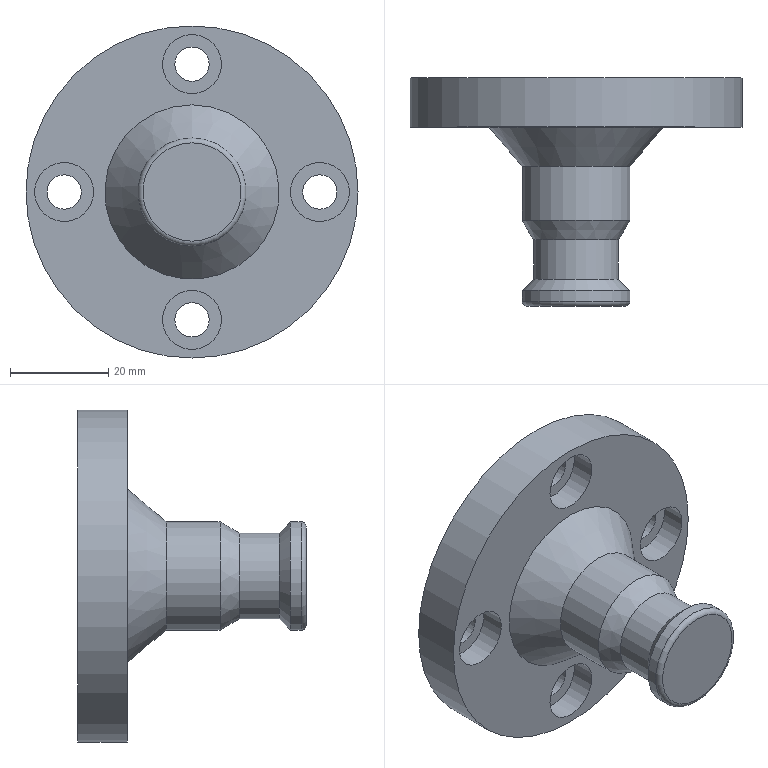Part | STEP file | Clamping device rod | 1 solid | 23 faces | box 67.5 x 46.39 x 67.5 mm | volume 47194 mm3 | cylinder 12 | plane 7 | cone 3 | torus 1 | commonest cylinder face diameters 7 x4 12 x4 22 x2 17.381 x1 67.5 x1
STEP:
#1=CARTESIAN_POINT('',(0.,38.89,-33.75));
#2=VERTEX_POINT('',#1);
#3=CARTESIAN_POINT('',(0.,38.89,0.));
#4=DIRECTION('',(0.,1.,0.));
#5=DIRECTION('',(0.,0.,-1.));
#6=AXIS2_PLACEMENT_3D('',#3,#4,#5);
#7=CIRCLE('',#6,33.75);
#8=EDGE_CURVE('',#2,#2,#7,.T.);
#9=ORIENTED_EDGE('',*,*,#8,.F.);
#10=EDGE_LOOP('',(#9));
#11=FACE_BOUND('',#10,.T.);
#12=CARTESIAN_POINT('',(26.,38.89,-6.));
#13=VERTEX_POINT('',#12);
#14=CARTESIAN_POINT('',(26.,38.89,0.));
#15=DIRECTION('',(0.,-1.,0.));
#16=DIRECTION('',(0.,0.,-1.));
#17=AXIS2_PLACEMENT_3D('',#14,#15,#16);
#18=CIRCLE('',#17,6.);
#19=EDGE_CURVE('',#13,#13,#18,.F.);
#20=ORIENTED_EDGE('',*,*,#19,.T.);
#21=EDGE_LOOP('',(#20));
#22=FACE_BOUND('',#21,.T.);
#23=CARTESIAN_POINT('',(-6.,38.89,-26.));
#24=VERTEX_POINT('',#23);
#25=CARTESIAN_POINT('',(0.,38.89,-26.));
#26=DIRECTION('',(0.,-1.,0.));
#27=DIRECTION('',(-1.,0.,0.));
#28=AXIS2_PLACEMENT_3D('',#25,#26,#27);
#29=CIRCLE('',#28,6.);
#30=EDGE_CURVE('',#24,#24,#29,.F.);
#31=ORIENTED_EDGE('',*,*,#30,.T.);
#32=EDGE_LOOP('',(#31));
#33=FACE_BOUND('',#32,.T.);
#34=CARTESIAN_POINT('',(-26.,38.89,6.));
#35=VERTEX_POINT('',#34);
#36=CARTESIAN_POINT('',(-26.,38.89,0.));
#37=DIRECTION('',(0.,-1.,0.));
#38=DIRECTION('',(0.,0.,1.));
#39=AXIS2_PLACEMENT_3D('',#36,#37,#38);
#40=CIRCLE('',#39,6.);
#41=EDGE_CURVE('',#35,#35,#40,.F.);
#42=ORIENTED_EDGE('',*,*,#41,.T.);
#43=EDGE_LOOP('',(#42));
#44=FACE_BOUND('',#43,.T.);
#45=CARTESIAN_POINT('',(0.,38.89,17.713));
#46=VERTEX_POINT('',#45);
#47=CARTESIAN_POINT('',(0.,38.89,0.));
#48=DIRECTION('',(0.,1.,0.));
#49=DIRECTION('',(0.,0.,1.));
#50=AXIS2_PLACEMENT_3D('',#47,#48,#49);
#51=CIRCLE('',#50,17.713);
#52=EDGE_CURVE('',#46,#46,#51,.T.);
#53=ORIENTED_EDGE('',*,*,#52,.T.);
#54=EDGE_LOOP('',(#53));
#55=FACE_BOUND('',#54,.T.);
#56=CARTESIAN_POINT('',(6.,38.89,26.));
#57=VERTEX_POINT('',#56);
#58=CARTESIAN_POINT('',(0.,38.89,26.));
#59=DIRECTION('',(0.,-1.,0.));
#60=DIRECTION('',(1.,0.,0.));
#61=AXIS2_PLACEMENT_3D('',#58,#59,#60);
#62=CIRCLE('',#61,6.);
#63=EDGE_CURVE('',#57,#57,#62,.F.);
#64=ORIENTED_EDGE('',*,*,#63,.T.);
#65=EDGE_LOOP('',(#64));
#66=FACE_BOUND('',#65,.T.);
#67=CARTESIAN_POINT('',(0.,38.89,0.));
#68=DIRECTION('',(0.,-1.,0.));
#69=DIRECTION('',(0.,0.,1.));
#70=AXIS2_PLACEMENT_3D('',#67,#68,#69);
#71=PLANE('',#70);
#72=ADVANCED_FACE('',(#11,#22,#33,#44,#55,#66),#71,.T.);
#73=CARTESIAN_POINT('',(0.,48.89,-33.75));
#74=VERTEX_POINT('',#73);
#75=CARTESIAN_POINT('',(0.,48.89,0.));
#76=DIRECTION('',(0.,1.,0.));
#77=DIRECTION('',(0.,0.,-1.));
#78=AXIS2_PLACEMENT_3D('',#75,#76,#77);
#79=CIRCLE('',#78,33.75);
#80=EDGE_CURVE('',#74,#74,#79,.T.);
#81=ORIENTED_EDGE('',*,*,#80,.T.);
#82=EDGE_LOOP('',(#81));
#83=FACE_BOUND('',#82,.T.);
#84=CARTESIAN_POINT('',(26.,48.89,-3.5));
#85=VERTEX_POINT('',#84);
#86=CARTESIAN_POINT('',(26.,48.89,0.));
#87=DIRECTION('',(0.,-1.,0.));
#88=DIRECTION('',(0.,0.,-1.));
#89=AXIS2_PLACEMENT_3D('',#86,#87,#88);
#90=CIRCLE('',#89,3.5);
#91=EDGE_CURVE('',#85,#85,#90,.T.);
#92=ORIENTED_EDGE('',*,*,#91,.T.);
#93=EDGE_LOOP('',(#92));
#94=FACE_BOUND('',#93,.T.);
#95=CARTESIAN_POINT('',(-3.5,48.89,-26.));
#96=VERTEX_POINT('',#95);
#97=CARTESIAN_POINT('',(0.,48.89,-26.));
#98=DIRECTION('',(0.,-1.,0.));
#99=DIRECTION('',(-1.,0.,0.));
#100=AXIS2_PLACEMENT_3D('',#97,#98,#99);
#101=CIRCLE('',#100,3.5);
#102=EDGE_CURVE('',#96,#96,#101,.T.);
#103=ORIENTED_EDGE('',*,*,#102,.T.);
#104=EDGE_LOOP('',(#103));
#105=FACE_BOUND('',#104,.T.);
#106=CARTESIAN_POINT('',(-26.,48.89,3.5));
#107=VERTEX_POINT('',#106);
#108=CARTESIAN_POINT('',(-26.,48.89,0.));
#109=DIRECTION('',(0.,-1.,0.));
#110=DIRECTION('',(0.,0.,1.));
#111=AXIS2_PLACEMENT_3D('',#108,#109,#110);
#112=CIRCLE('',#111,3.5);
#113=EDGE_CURVE('',#107,#107,#112,.T.);
#114=ORIENTED_EDGE('',*,*,#113,.T.);
#115=EDGE_LOOP('',(#114));
#116=FACE_BOUND('',#115,.T.);
#117=CARTESIAN_POINT('',(3.5,48.89,26.));
#118=VERTEX_POINT('',#117);
#119=CARTESIAN_POINT('',(0.,48.89,26.));
#120=DIRECTION('',(0.,-1.,0.));
#121=DIRECTION('',(1.,0.,0.));
#122=AXIS2_PLACEMENT_3D('',#119,#120,#121);
#123=CIRCLE('',#122,3.5);
#124=EDGE_CURVE('',#118,#118,#123,.T.);
#125=ORIENTED_EDGE('',*,*,#124,.T.);
#126=EDGE_LOOP('',(#125));
#127=FACE_BOUND('',#126,.T.);
#128=CARTESIAN_POINT('',(0.,48.89,0.));
#129=DIRECTION('',(0.,1.,0.));
#130=DIRECTION('',(0.,0.,1.));
#131=AXIS2_PLACEMENT_3D('',#128,#129,#130);
#132=PLANE('',#131);
#133=ADVANCED_FACE('',(#83,#94,#105,#116,#127),#132,.T.);
#134=ORIENTED_EDGE('',*,*,#80,.F.);
#135=EDGE_LOOP('',(#134));
#136=FACE_OUTER_BOUND('',#135,.T.);
#137=ORIENTED_EDGE('',*,*,#8,.T.);
#138=EDGE_LOOP('',(#137));
#139=FACE_OUTER_BOUND('',#138,.T.);
#140=CARTESIAN_POINT('',(0.,38.89,0.));
#141=DIRECTION('',(0.,1.,0.));
#142=DIRECTION('',(0.,0.,-1.));
#143=AXIS2_PLACEMENT_3D('',#140,#141,#142);
#144=CYLINDRICAL_SURFACE('',#143,33.75);
#145=ADVANCED_FACE('',(#136,#139),#144,.T.);
#146=CARTESIAN_POINT('',(26.,43.89,-6.));
#147=VERTEX_POINT('',#146);
#148=CARTESIAN_POINT('',(26.,43.89,0.));
#149=DIRECTION('',(0.,-1.,0.));
#150=DIRECTION('',(0.,0.,-1.));
#151=AXIS2_PLACEMENT_3D('',#148,#149,#150);
#152=CIRCLE('',#151,6.);
#153=EDGE_CURVE('',#147,#147,#152,.T.);
#154=ORIENTED_EDGE('',*,*,#153,.F.);
#155=EDGE_LOOP('',(#154));
#156=FACE_OUTER_BOUND('',#155,.T.);
#157=ORIENTED_EDGE('',*,*,#19,.F.);
#158=EDGE_LOOP('',(#157));
#159=FACE_OUTER_BOUND('',#158,.T.);
#160=CARTESIAN_POINT('',(26.,43.89,0.));
#161=DIRECTION('',(0.,-1.,0.));
#162=DIRECTION('',(0.,0.,-1.));
#163=AXIS2_PLACEMENT_3D('',#160,#161,#162);
#164=CYLINDRICAL_SURFACE('',#163,6.);
#165=ADVANCED_FACE('',(#156,#159),#164,.F.);
#166=CARTESIAN_POINT('',(-6.,43.89,-26.));
#167=VERTEX_POINT('',#166);
#168=CARTESIAN_POINT('',(0.,43.89,-26.));
#169=DIRECTION('',(0.,-1.,0.));
#170=DIRECTION('',(-1.,0.,0.));
#171=AXIS2_PLACEMENT_3D('',#168,#169,#170);
#172=CIRCLE('',#171,6.);
#173=EDGE_CURVE('',#167,#167,#172,.T.);
#174=ORIENTED_EDGE('',*,*,#173,.F.);
#175=EDGE_LOOP('',(#174));
#176=FACE_OUTER_BOUND('',#175,.T.);
#177=ORIENTED_EDGE('',*,*,#30,.F.);
#178=EDGE_LOOP('',(#177));
#179=FACE_OUTER_BOUND('',#178,.T.);
#180=CARTESIAN_POINT('',(0.,43.89,-26.));
#181=DIRECTION('',(0.,-1.,0.));
#182=DIRECTION('',(-1.,0.,0.));
#183=AXIS2_PLACEMENT_3D('',#180,#181,#182);
#184=CYLINDRICAL_SURFACE('',#183,6.);
#185=ADVANCED_FACE('',(#176,#179),#184,.F.);
#186=CARTESIAN_POINT('',(-26.,43.89,6.));
#187=VERTEX_POINT('',#186);
#188=CARTESIAN_POINT('',(-26.,43.89,0.));
#189=DIRECTION('',(0.,-1.,0.));
#190=DIRECTION('',(0.,0.,1.));
#191=AXIS2_PLACEMENT_3D('',#188,#189,#190);
#192=CIRCLE('',#191,6.);
#193=EDGE_CURVE('',#187,#187,#192,.T.);
#194=ORIENTED_EDGE('',*,*,#193,.F.);
#195=EDGE_LOOP('',(#194));
#196=FACE_OUTER_BOUND('',#195,.T.);
#197=ORIENTED_EDGE('',*,*,#41,.F.);
#198=EDGE_LOOP('',(#197));
#199=FACE_OUTER_BOUND('',#198,.T.);
#200=CARTESIAN_POINT('',(-26.,43.89,0.));
#201=DIRECTION('',(0.,-1.,0.));
#202=DIRECTION('',(0.,0.,1.));
#203=AXIS2_PLACEMENT_3D('',#200,#201,#202);
#204=CYLINDRICAL_SURFACE('',#203,6.);
#205=ADVANCED_FACE('',(#196,#199),#204,.F.);
#206=ORIENTED_EDGE('',*,*,#52,.F.);
#207=EDGE_LOOP('',(#206));
#208=FACE_OUTER_BOUND('',#207,.T.);
#209=CARTESIAN_POINT('',(0.,30.89,11.));
#210=VERTEX_POINT('',#209);
#211=CARTESIAN_POINT('',(0.,30.89,0.));
#212=DIRECTION('',(0.,1.,0.));
#213=DIRECTION('',(0.,0.,1.));
#214=AXIS2_PLACEMENT_3D('',#211,#212,#213);
#215=CIRCLE('',#214,11.);
#216=EDGE_CURVE('',#210,#210,#215,.T.);
#217=ORIENTED_EDGE('',*,*,#216,.T.);
#218=EDGE_LOOP('',(#217));
#219=FACE_OUTER_BOUND('',#218,.T.);
#220=CARTESIAN_POINT('',(0.,34.89,0.));
#221=DIRECTION('',(0.,1.,0.));
#222=DIRECTION('',(0.,0.,1.));
#223=AXIS2_PLACEMENT_3D('',#220,#221,#222);
#224=CONICAL_SURFACE('',#223,14.356,0.6981);
#225=ADVANCED_FACE('',(#208,#219),#224,.T.);
#226=CARTESIAN_POINT('',(6.,43.89,26.));
#227=VERTEX_POINT('',#226);
#228=CARTESIAN_POINT('',(0.,43.89,26.));
#229=DIRECTION('',(0.,-1.,0.));
#230=DIRECTION('',(1.,0.,0.));
#231=AXIS2_PLACEMENT_3D('',#228,#229,#230);
#232=CIRCLE('',#231,6.);
#233=EDGE_CURVE('',#227,#227,#232,.T.);
#234=ORIENTED_EDGE('',*,*,#233,.F.);
#235=EDGE_LOOP('',(#234));
#236=FACE_OUTER_BOUND('',#235,.T.);
#237=ORIENTED_EDGE('',*,*,#63,.F.);
#238=EDGE_LOOP('',(#237));
#239=FACE_OUTER_BOUND('',#238,.T.);
#240=CARTESIAN_POINT('',(0.,43.89,26.));
#241=DIRECTION('',(0.,-1.,0.));
#242=DIRECTION('',(1.,0.,0.));
#243=AXIS2_PLACEMENT_3D('',#240,#241,#242);
#244=CYLINDRICAL_SURFACE('',#243,6.);
#245=ADVANCED_FACE('',(#236,#239),#244,.F.);
#246=ORIENTED_EDGE('',*,*,#91,.F.);
#247=EDGE_LOOP('',(#246));
#248=FACE_OUTER_BOUND('',#247,.T.);
#249=CARTESIAN_POINT('',(26.,43.89,-3.5));
#250=VERTEX_POINT('',#249);
#251=CARTESIAN_POINT('',(26.,43.89,0.));
#252=DIRECTION('',(0.,-1.,0.));
#253=DIRECTION('',(0.,0.,-1.));
#254=AXIS2_PLACEMENT_3D('',#251,#252,#253);
#255=CIRCLE('',#254,3.5);
#256=EDGE_CURVE('',#250,#250,#255,.T.);
#257=ORIENTED_EDGE('',*,*,#256,.T.);
#258=EDGE_LOOP('',(#257));
#259=FACE_OUTER_BOUND('',#258,.T.);
#260=CARTESIAN_POINT('',(26.,78.89,0.));
#261=DIRECTION('',(0.,-1.,0.));
#262=DIRECTION('',(0.,0.,-1.));
#263=AXIS2_PLACEMENT_3D('',#260,#261,#262);
#264=CYLINDRICAL_SURFACE('',#263,3.5);
#265=ADVANCED_FACE('',(#248,#259),#264,.F.);
#266=ORIENTED_EDGE('',*,*,#102,.F.);
#267=EDGE_LOOP('',(#266));
#268=FACE_OUTER_BOUND('',#267,.T.);
#269=CARTESIAN_POINT('',(-3.5,43.89,-26.));
#270=VERTEX_POINT('',#269);
#271=CARTESIAN_POINT('',(0.,43.89,-26.));
#272=DIRECTION('',(0.,-1.,0.));
#273=DIRECTION('',(-1.,0.,0.));
#274=AXIS2_PLACEMENT_3D('',#271,#272,#273);
#275=CIRCLE('',#274,3.5);
#276=EDGE_CURVE('',#270,#270,#275,.T.);
#277=ORIENTED_EDGE('',*,*,#276,.T.);
#278=EDGE_LOOP('',(#277));
#279=FACE_OUTER_BOUND('',#278,.T.);
#280=CARTESIAN_POINT('',(0.,78.89,-26.));
#281=DIRECTION('',(0.,-1.,0.));
#282=DIRECTION('',(-1.,0.,0.));
#283=AXIS2_PLACEMENT_3D('',#280,#281,#282);
#284=CYLINDRICAL_SURFACE('',#283,3.5);
#285=ADVANCED_FACE('',(#268,#279),#284,.F.);
#286=ORIENTED_EDGE('',*,*,#113,.F.);
#287=EDGE_LOOP('',(#286));
#288=FACE_OUTER_BOUND('',#287,.T.);
#289=CARTESIAN_POINT('',(-26.,43.89,3.5));
#290=VERTEX_POINT('',#289);
#291=CARTESIAN_POINT('',(-26.,43.89,0.));
#292=DIRECTION('',(0.,-1.,0.));
#293=DIRECTION('',(0.,0.,1.));
#294=AXIS2_PLACEMENT_3D('',#291,#292,#293);
#295=CIRCLE('',#294,3.5);
#296=EDGE_CURVE('',#290,#290,#295,.T.);
#297=ORIENTED_EDGE('',*,*,#296,.T.);
#298=EDGE_LOOP('',(#297));
#299=FACE_OUTER_BOUND('',#298,.T.);
#300=CARTESIAN_POINT('',(-26.,78.89,0.));
#301=DIRECTION('',(0.,-1.,0.));
#302=DIRECTION('',(0.,0.,1.));
#303=AXIS2_PLACEMENT_3D('',#300,#301,#302);
#304=CYLINDRICAL_SURFACE('',#303,3.5);
#305=ADVANCED_FACE('',(#288,#299),#304,.F.);
#306=ORIENTED_EDGE('',*,*,#124,.F.);
#307=EDGE_LOOP('',(#306));
#308=FACE_OUTER_BOUND('',#307,.T.);
#309=CARTESIAN_POINT('',(3.5,43.89,26.));
#310=VERTEX_POINT('',#309);
#311=CARTESIAN_POINT('',(0.,43.89,26.));
#312=DIRECTION('',(0.,-1.,0.));
#313=DIRECTION('',(1.,0.,0.));
#314=AXIS2_PLACEMENT_3D('',#311,#312,#313);
#315=CIRCLE('',#314,3.5);
#316=EDGE_CURVE('',#310,#310,#315,.T.);
#317=ORIENTED_EDGE('',*,*,#316,.T.);
#318=EDGE_LOOP('',(#317));
#319=FACE_OUTER_BOUND('',#318,.T.);
#320=CARTESIAN_POINT('',(0.,78.89,26.));
#321=DIRECTION('',(0.,-1.,0.));
#322=DIRECTION('',(1.,0.,0.));
#323=AXIS2_PLACEMENT_3D('',#320,#321,#322);
#324=CYLINDRICAL_SURFACE('',#323,3.5);
#325=ADVANCED_FACE('',(#308,#319),#324,.F.);
#326=ORIENTED_EDGE('',*,*,#153,.T.);
#327=EDGE_LOOP('',(#326));
#328=FACE_BOUND('',#327,.T.);
#329=ORIENTED_EDGE('',*,*,#256,.F.);
#330=EDGE_LOOP('',(#329));
#331=FACE_BOUND('',#330,.T.);
#332=CARTESIAN_POINT('',(26.,43.89,0.));
#333=DIRECTION('',(0.,1.,0.));
#334=DIRECTION('',(0.,0.,-1.));
#335=AXIS2_PLACEMENT_3D('',#332,#333,#334);
#336=PLANE('',#335);
#337=ADVANCED_FACE('',(#328,#331),#336,.F.);
#338=ORIENTED_EDGE('',*,*,#173,.T.);
#339=EDGE_LOOP('',(#338));
#340=FACE_BOUND('',#339,.T.);
#341=ORIENTED_EDGE('',*,*,#276,.F.);
#342=EDGE_LOOP('',(#341));
#343=FACE_BOUND('',#342,.T.);
#344=CARTESIAN_POINT('',(0.,43.89,-26.));
#345=DIRECTION('',(0.,1.,0.));
#346=DIRECTION('',(-1.,0.,0.));
#347=AXIS2_PLACEMENT_3D('',#344,#345,#346);
#348=PLANE('',#347);
#349=ADVANCED_FACE('',(#340,#343),#348,.F.);
#350=ORIENTED_EDGE('',*,*,#193,.T.);
#351=EDGE_LOOP('',(#350));
#352=FACE_BOUND('',#351,.T.);
#353=ORIENTED_EDGE('',*,*,#296,.F.);
#354=EDGE_LOOP('',(#353));
#355=FACE_BOUND('',#354,.T.);
#356=CARTESIAN_POINT('',(-26.,43.89,0.));
#357=DIRECTION('',(0.,1.,0.));
#358=DIRECTION('',(0.,0.,1.));
#359=AXIS2_PLACEMENT_3D('',#356,#357,#358);
#360=PLANE('',#359);
#361=ADVANCED_FACE('',(#352,#355),#360,.F.);
#362=ORIENTED_EDGE('',*,*,#216,.F.);
#363=EDGE_LOOP('',(#362));
#364=FACE_OUTER_BOUND('',#363,.T.);
#365=CARTESIAN_POINT('',(0.,20.,11.));
#366=VERTEX_POINT('',#365);
#367=CARTESIAN_POINT('',(0.,20.,0.));
#368=DIRECTION('',(0.,1.,0.));
#369=DIRECTION('',(0.,0.,1.));
#370=AXIS2_PLACEMENT_3D('',#367,#368,#369);
#371=CIRCLE('',#370,11.);
#372=EDGE_CURVE('',#366,#366,#371,.T.);
#373=ORIENTED_EDGE('',*,*,#372,.T.);
#374=EDGE_LOOP('',(#373));
#375=FACE_OUTER_BOUND('',#374,.T.);
#376=CARTESIAN_POINT('',(0.,20.,0.));
#377=DIRECTION('',(0.,1.,0.));
#378=DIRECTION('',(0.,0.,1.));
#379=AXIS2_PLACEMENT_3D('',#376,#377,#378);
#380=CYLINDRICAL_SURFACE('',#379,11.);
#381=ADVANCED_FACE('',(#364,#375),#380,.T.);
#382=ORIENTED_EDGE('',*,*,#233,.T.);
#383=EDGE_LOOP('',(#382));
#384=FACE_BOUND('',#383,.T.);
#385=ORIENTED_EDGE('',*,*,#316,.F.);
#386=EDGE_LOOP('',(#385));
#387=FACE_BOUND('',#386,.T.);
#388=CARTESIAN_POINT('',(0.,43.89,26.));
#389=DIRECTION('',(0.,1.,0.));
#390=DIRECTION('',(1.,0.,0.));
#391=AXIS2_PLACEMENT_3D('',#388,#389,#390);
#392=PLANE('',#391);
#393=ADVANCED_FACE('',(#384,#387),#392,.F.);
#394=ORIENTED_EDGE('',*,*,#372,.F.);
#395=EDGE_LOOP('',(#394));
#396=FACE_OUTER_BOUND('',#395,.T.);
#397=CARTESIAN_POINT('',(0.,16.,8.691));
#398=VERTEX_POINT('',#397);
#399=CARTESIAN_POINT('',(0.,16.,0.));
#400=DIRECTION('',(0.,1.,0.));
#401=DIRECTION('',(0.,0.,1.));
#402=AXIS2_PLACEMENT_3D('',#399,#400,#401);
#403=CIRCLE('',#402,8.691);
#404=EDGE_CURVE('',#398,#398,#403,.T.);
#405=ORIENTED_EDGE('',*,*,#404,.T.);
#406=EDGE_LOOP('',(#405));
#407=FACE_OUTER_BOUND('',#406,.T.);
#408=CARTESIAN_POINT('',(0.,18.,0.));
#409=DIRECTION('',(0.,1.,0.));
#410=DIRECTION('',(0.,0.,1.));
#411=AXIS2_PLACEMENT_3D('',#408,#409,#410);
#412=CONICAL_SURFACE('',#411,9.845,0.5236);
#413=ADVANCED_FACE('',(#396,#407),#412,.T.);
#414=ORIENTED_EDGE('',*,*,#404,.F.);
#415=EDGE_LOOP('',(#414));
#416=FACE_OUTER_BOUND('',#415,.T.);
#417=CARTESIAN_POINT('',(0.,8.,8.691));
#418=VERTEX_POINT('',#417);
#419=CARTESIAN_POINT('',(0.,8.,0.));
#420=DIRECTION('',(0.,1.,0.));
#421=DIRECTION('',(0.,0.,1.));
#422=AXIS2_PLACEMENT_3D('',#419,#420,#421);
#423=CIRCLE('',#422,8.691);
#424=EDGE_CURVE('',#418,#418,#423,.T.);
#425=ORIENTED_EDGE('',*,*,#424,.T.);
#426=EDGE_LOOP('',(#425));
#427=FACE_OUTER_BOUND('',#426,.T.);
#428=CARTESIAN_POINT('',(0.,8.,0.));
#429=DIRECTION('',(0.,1.,0.));
#430=DIRECTION('',(0.,0.,1.));
#431=AXIS2_PLACEMENT_3D('',#428,#429,#430);
#432=CYLINDRICAL_SURFACE('',#431,8.691);
#433=ADVANCED_FACE('',(#416,#427),#432,.T.);
#434=ORIENTED_EDGE('',*,*,#424,.F.);
#435=EDGE_LOOP('',(#434));
#436=FACE_OUTER_BOUND('',#435,.T.);
#437=CARTESIAN_POINT('',(0.,5.691,11.));
#438=VERTEX_POINT('',#437);
#439=CARTESIAN_POINT('',(0.,5.691,0.));
#440=DIRECTION('',(0.,1.,0.));
#441=DIRECTION('',(0.,0.,1.));
#442=AXIS2_PLACEMENT_3D('',#439,#440,#441);
#443=CIRCLE('',#442,11.);
#444=EDGE_CURVE('',#438,#438,#443,.T.);
#445=ORIENTED_EDGE('',*,*,#444,.T.);
#446=EDGE_LOOP('',(#445));
#447=FACE_OUTER_BOUND('',#446,.T.);
#448=CARTESIAN_POINT('',(0.,6.845,0.));
#449=DIRECTION('',(0.,-1.,0.));
#450=DIRECTION('',(0.,0.,-1.));
#451=AXIS2_PLACEMENT_3D('',#448,#449,#450);
#452=CONICAL_SURFACE('',#451,9.845,0.7854);
#453=ADVANCED_FACE('',(#436,#447),#452,.T.);
#454=ORIENTED_EDGE('',*,*,#444,.F.);
#455=EDGE_LOOP('',(#454));
#456=FACE_OUTER_BOUND('',#455,.T.);
#457=CARTESIAN_POINT('',(0.,3.5,11.));
#458=VERTEX_POINT('',#457);
#459=CARTESIAN_POINT('',(0.,3.5,0.));
#460=DIRECTION('',(0.,1.,0.));
#461=DIRECTION('',(0.,0.,1.));
#462=AXIS2_PLACEMENT_3D('',#459,#460,#461);
#463=CIRCLE('',#462,11.);
#464=EDGE_CURVE('',#458,#458,#463,.F.);
#465=ORIENTED_EDGE('',*,*,#464,.F.);
#466=EDGE_LOOP('',(#465));
#467=FACE_OUTER_BOUND('',#466,.T.);
#468=CARTESIAN_POINT('',(0.,20.,0.));
#469=DIRECTION('',(0.,1.,0.));
#470=DIRECTION('',(0.,0.,1.));
#471=AXIS2_PLACEMENT_3D('',#468,#469,#470);
#472=CYLINDRICAL_SURFACE('',#471,11.);
#473=ADVANCED_FACE('',(#456,#467),#472,.T.);
#474=ORIENTED_EDGE('',*,*,#464,.T.);
#475=EDGE_LOOP('',(#474));
#476=FACE_OUTER_BOUND('',#475,.T.);
#477=CARTESIAN_POINT('',(0.,2.5,10.));
#478=VERTEX_POINT('',#477);
#479=CARTESIAN_POINT('',(0.,2.5,0.));
#480=DIRECTION('',(0.,1.,0.));
#481=DIRECTION('',(0.,0.,1.));
#482=AXIS2_PLACEMENT_3D('',#479,#480,#481);
#483=CIRCLE('',#482,10.);
#484=EDGE_CURVE('',#478,#478,#483,.F.);
#485=ORIENTED_EDGE('',*,*,#484,.F.);
#486=EDGE_LOOP('',(#485));
#487=FACE_OUTER_BOUND('',#486,.T.);
#488=CARTESIAN_POINT('',(0.,3.5,0.));
#489=DIRECTION('',(0.,1.,0.));
#490=DIRECTION('',(0.,0.,1.));
#491=AXIS2_PLACEMENT_3D('',#488,#489,#490);
#492=TOROIDAL_SURFACE('',#491,10.,1.);
#493=ADVANCED_FACE('',(#476,#487),#492,.T.);
#494=ORIENTED_EDGE('',*,*,#484,.T.);
#495=EDGE_LOOP('',(#494));
#496=FACE_BOUND('',#495,.T.);
#497=CARTESIAN_POINT('',(-50.,2.5,-13.799));
#498=DIRECTION('',(0.,1.,0.));
#499=DIRECTION('',(0.,0.,1.));
#500=AXIS2_PLACEMENT_3D('',#497,#498,#499);
#501=PLANE('',#500);
#502=ADVANCED_FACE('',(#496),#501,.F.);
#503=CLOSED_SHELL('',(#72,#133,#145,#165,#185,#205,#225,#245,#265,#285,#305,#325,#337,#349,#361,#381,#393,#413,#433,#453,#473,#493,#502));
#504=MANIFOLD_SOLID_BREP('',#503);
#505=(LENGTH_UNIT()NAMED_UNIT(*)SI_UNIT(.MILLI.,.METRE.));
#506=UNCERTAINTY_MEASURE_WITH_UNIT(LENGTH_MEASURE(0.00001),#505,'','');
#507=(NAMED_UNIT(*)PLANE_ANGLE_UNIT()SI_UNIT($,.RADIAN.));
#508=(NAMED_UNIT(*)SI_UNIT($,.STERADIAN.)SOLID_ANGLE_UNIT());
#509=(GEOMETRIC_REPRESENTATION_CONTEXT(3)GLOBAL_UNCERTAINTY_ASSIGNED_CONTEXT((#506))GLOBAL_UNIT_ASSIGNED_CONTEXT((#505,#507,#508))REPRESENTATION_CONTEXT('',''));
#510=ADVANCED_BREP_SHAPE_REPRESENTATION('',(#504),#509);